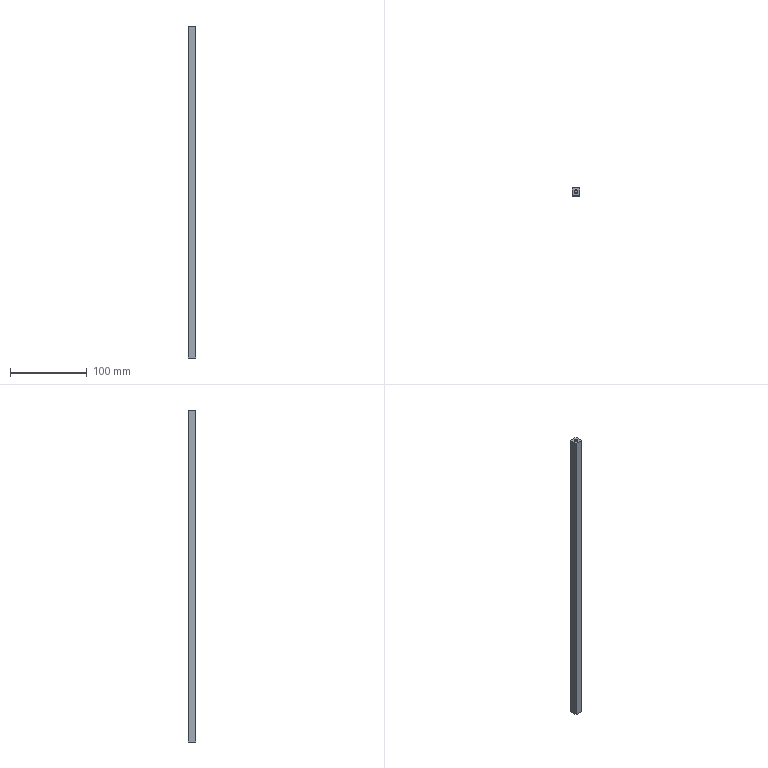Part | STEP file | End strip | 1 solid | 16 faces | box 10 x 10 x 432 mm | volume 42976 mm3 | plane 8 | cone 4 | cylinder 4 | commonest cylinder face diameters 3 x4
STEP:
#1=CARTESIAN_POINT('',(-16.382,-19.086,1.));
#2=VERTEX_POINT('',#1);
#3=CARTESIAN_POINT('',(-19.382,-19.086,1.));
#4=VERTEX_POINT('',#3);
#5=CARTESIAN_POINT('',(-17.882,-19.086,1.));
#6=DIRECTION('',(0.,0.,-1.));
#7=DIRECTION('',(-1.,0.,0.));
#8=AXIS2_PLACEMENT_3D('',#5,#6,#7);
#9=CIRCLE('',#8,1.5);
#10=EDGE_CURVE('',#2,#4,#9,.T.);
#11=ORIENTED_EDGE('',*,*,#10,.F.);
#12=CARTESIAN_POINT('',(-15.382,-19.086,0.));
#13=VERTEX_POINT('',#12);
#14=CARTESIAN_POINT('',(-15.382,-19.086,0.));
#15=DIRECTION('',(0.7071,0.,-0.7071));
#16=VECTOR('',#15,1000.);
#17=LINE('',#14,#16);
#18=EDGE_CURVE('',#2,#13,#17,.T.);
#19=ORIENTED_EDGE('',*,*,#18,.T.);
#20=CARTESIAN_POINT('',(-20.382,-19.086,0.));
#21=VERTEX_POINT('',#20);
#22=CARTESIAN_POINT('',(-17.882,-19.086,0.));
#23=DIRECTION('',(0.,0.,-1.));
#24=DIRECTION('',(-1.,0.,0.));
#25=AXIS2_PLACEMENT_3D('',#22,#23,#24);
#26=CIRCLE('',#25,2.5);
#27=EDGE_CURVE('',#13,#21,#26,.T.);
#28=ORIENTED_EDGE('',*,*,#27,.T.);
#29=CARTESIAN_POINT('',(-20.382,-19.086,0.));
#30=DIRECTION('',(-0.7071,0.,-0.7071));
#31=VECTOR('',#30,1000.);
#32=LINE('',#29,#31);
#33=EDGE_CURVE('',#4,#21,#32,.T.);
#34=ORIENTED_EDGE('',*,*,#33,.F.);
#35=EDGE_LOOP('',(#11,#19,#28,#34));
#36=FACE_OUTER_BOUND('',#35,.T.);
#37=CARTESIAN_POINT('',(-17.882,-19.086,0.));
#38=DIRECTION('',(0.,0.,-1.));
#39=DIRECTION('',(-1.,0.,0.));
#40=AXIS2_PLACEMENT_3D('',#37,#38,#39);
#41=CONICAL_SURFACE('',#40,2.5,0.7854);
#42=ADVANCED_FACE('',(#36),#41,.F.);
#43=CARTESIAN_POINT('',(-17.882,-17.586,431.));
#44=VERTEX_POINT('',#43);
#45=CARTESIAN_POINT('',(-19.382,-19.086,431.));
#46=VERTEX_POINT('',#45);
#47=CARTESIAN_POINT('',(-17.882,-19.086,431.));
#48=DIRECTION('',(0.,0.,1.));
#49=DIRECTION('',(1.,0.,0.));
#50=AXIS2_PLACEMENT_3D('',#47,#48,#49);
#51=CIRCLE('',#50,1.5);
#52=EDGE_CURVE('',#44,#46,#51,.T.);
#53=ORIENTED_EDGE('',*,*,#52,.F.);
#54=CARTESIAN_POINT('',(-17.882,-16.586,432.));
#55=VERTEX_POINT('',#54);
#56=CARTESIAN_POINT('',(-17.882,-16.586,432.));
#57=DIRECTION('',(0.,0.7071,0.7071));
#58=VECTOR('',#57,1000.);
#59=LINE('',#56,#58);
#60=EDGE_CURVE('',#44,#55,#59,.T.);
#61=ORIENTED_EDGE('',*,*,#60,.T.);
#62=CARTESIAN_POINT('',(-17.882,-21.586,432.));
#63=VERTEX_POINT('',#62);
#64=CARTESIAN_POINT('',(-17.882,-19.086,432.));
#65=DIRECTION('',(0.,0.,-1.));
#66=DIRECTION('',(0.,-1.,0.));
#67=AXIS2_PLACEMENT_3D('',#64,#65,#66);
#68=CIRCLE('',#67,2.5);
#69=EDGE_CURVE('',#63,#55,#68,.T.);
#70=ORIENTED_EDGE('',*,*,#69,.F.);
#71=CARTESIAN_POINT('',(-17.882,-20.586,431.));
#72=VERTEX_POINT('',#71);
#73=CARTESIAN_POINT('',(-17.882,-21.586,432.));
#74=DIRECTION('',(0.,-0.7071,0.7071));
#75=VECTOR('',#74,1000.);
#76=LINE('',#73,#75);
#77=EDGE_CURVE('',#72,#63,#76,.T.);
#78=ORIENTED_EDGE('',*,*,#77,.F.);
#79=CARTESIAN_POINT('',(-17.882,-19.086,431.));
#80=DIRECTION('',(0.,0.,1.));
#81=DIRECTION('',(1.,0.,0.));
#82=AXIS2_PLACEMENT_3D('',#79,#80,#81);
#83=CIRCLE('',#82,1.5);
#84=EDGE_CURVE('',#46,#72,#83,.T.);
#85=ORIENTED_EDGE('',*,*,#84,.F.);
#86=EDGE_LOOP('',(#53,#61,#70,#78,#85));
#87=FACE_OUTER_BOUND('',#86,.T.);
#88=CARTESIAN_POINT('',(-17.882,-19.086,432.));
#89=DIRECTION('',(0.,0.,1.));
#90=DIRECTION('',(0.,-1.,0.));
#91=AXIS2_PLACEMENT_3D('',#88,#89,#90);
#92=CONICAL_SURFACE('',#91,2.5,0.7854);
#93=ADVANCED_FACE('',(#87),#92,.F.);
#94=CARTESIAN_POINT('',(-16.382,-19.086,15.));
#95=VERTEX_POINT('',#94);
#96=CARTESIAN_POINT('',(-19.382,-19.086,15.));
#97=VERTEX_POINT('',#96);
#98=CARTESIAN_POINT('',(-17.882,-19.086,15.));
#99=DIRECTION('',(0.,0.,-1.));
#100=DIRECTION('',(-1.,0.,0.));
#101=AXIS2_PLACEMENT_3D('',#98,#99,#100);
#102=CIRCLE('',#101,1.5);
#103=EDGE_CURVE('',#95,#97,#102,.T.);
#104=ORIENTED_EDGE('',*,*,#103,.F.);
#105=CARTESIAN_POINT('',(-16.382,-19.086,15.));
#106=DIRECTION('',(0.,0.,-1.));
#107=VECTOR('',#106,1000.);
#108=LINE('',#105,#107);
#109=EDGE_CURVE('',#95,#2,#108,.T.);
#110=ORIENTED_EDGE('',*,*,#109,.T.);
#111=ORIENTED_EDGE('',*,*,#10,.T.);
#112=CARTESIAN_POINT('',(-19.382,-19.086,15.));
#113=DIRECTION('',(0.,0.,-1.));
#114=VECTOR('',#113,1000.);
#115=LINE('',#112,#114);
#116=EDGE_CURVE('',#97,#4,#115,.T.);
#117=ORIENTED_EDGE('',*,*,#116,.F.);
#118=EDGE_LOOP('',(#104,#110,#111,#117));
#119=FACE_OUTER_BOUND('',#118,.T.);
#120=CARTESIAN_POINT('',(-17.882,-19.086,15.));
#121=DIRECTION('',(0.,0.,-1.));
#122=DIRECTION('',(-1.,0.,0.));
#123=AXIS2_PLACEMENT_3D('',#120,#121,#122);
#124=CYLINDRICAL_SURFACE('',#123,1.5);
#125=ADVANCED_FACE('',(#119),#124,.F.);
#126=CARTESIAN_POINT('',(-19.382,-19.086,417.));
#127=VERTEX_POINT('',#126);
#128=CARTESIAN_POINT('',(-16.382,-19.086,417.));
#129=VERTEX_POINT('',#128);
#130=CARTESIAN_POINT('',(-17.882,-19.086,417.));
#131=DIRECTION('',(0.,0.,1.));
#132=DIRECTION('',(1.,0.,0.));
#133=AXIS2_PLACEMENT_3D('',#130,#131,#132);
#134=CIRCLE('',#133,1.5);
#135=EDGE_CURVE('',#127,#129,#134,.T.);
#136=ORIENTED_EDGE('',*,*,#135,.F.);
#137=CARTESIAN_POINT('',(-19.382,-19.086,417.));
#138=DIRECTION('',(0.,0.,1.));
#139=VECTOR('',#138,1000.);
#140=LINE('',#137,#139);
#141=EDGE_CURVE('',#127,#46,#140,.T.);
#142=ORIENTED_EDGE('',*,*,#141,.T.);
#143=ORIENTED_EDGE('',*,*,#84,.T.);
#144=CARTESIAN_POINT('',(-16.382,-19.086,431.));
#145=VERTEX_POINT('',#144);
#146=CARTESIAN_POINT('',(-17.882,-19.086,431.));
#147=DIRECTION('',(0.,0.,1.));
#148=DIRECTION('',(1.,0.,0.));
#149=AXIS2_PLACEMENT_3D('',#146,#147,#148);
#150=CIRCLE('',#149,1.5);
#151=EDGE_CURVE('',#72,#145,#150,.T.);
#152=ORIENTED_EDGE('',*,*,#151,.T.);
#153=CARTESIAN_POINT('',(-16.382,-19.086,417.));
#154=DIRECTION('',(0.,0.,1.));
#155=VECTOR('',#154,1000.);
#156=LINE('',#153,#155);
#157=EDGE_CURVE('',#129,#145,#156,.T.);
#158=ORIENTED_EDGE('',*,*,#157,.F.);
#159=EDGE_LOOP('',(#136,#142,#143,#152,#158));
#160=FACE_OUTER_BOUND('',#159,.T.);
#161=CARTESIAN_POINT('',(-17.882,-19.086,417.));
#162=DIRECTION('',(0.,0.,1.));
#163=DIRECTION('',(1.,0.,0.));
#164=AXIS2_PLACEMENT_3D('',#161,#162,#163);
#165=CYLINDRICAL_SURFACE('',#164,1.5);
#166=ADVANCED_FACE('',(#160),#165,.F.);
#167=CARTESIAN_POINT('',(-22.882,-24.086,432.));
#168=VERTEX_POINT('',#167);
#169=CARTESIAN_POINT('',(-22.882,-24.086,0.));
#170=VERTEX_POINT('',#169);
#171=CARTESIAN_POINT('',(-22.882,-24.086,432.));
#172=DIRECTION('',(0.,0.,-1.));
#173=VECTOR('',#172,1000.);
#174=LINE('',#171,#173);
#175=EDGE_CURVE('',#168,#170,#174,.T.);
#176=ORIENTED_EDGE('',*,*,#175,.F.);
#177=CARTESIAN_POINT('',(-22.882,-14.086,432.));
#178=VERTEX_POINT('',#177);
#179=CARTESIAN_POINT('',(-22.882,-14.086,432.));
#180=DIRECTION('',(0.,-1.,0.));
#181=VECTOR('',#180,1000.);
#182=LINE('',#179,#181);
#183=EDGE_CURVE('',#178,#168,#182,.T.);
#184=ORIENTED_EDGE('',*,*,#183,.F.);
#185=CARTESIAN_POINT('',(-22.882,-14.086,0.));
#186=VERTEX_POINT('',#185);
#187=CARTESIAN_POINT('',(-22.882,-14.086,432.));
#188=DIRECTION('',(0.,0.,1.));
#189=VECTOR('',#188,1000.);
#190=LINE('',#187,#189);
#191=EDGE_CURVE('',#186,#178,#190,.T.);
#192=ORIENTED_EDGE('',*,*,#191,.F.);
#193=CARTESIAN_POINT('',(-22.882,-14.086,0.));
#194=DIRECTION('',(0.,1.,0.));
#195=VECTOR('',#194,1000.);
#196=LINE('',#193,#195);
#197=EDGE_CURVE('',#170,#186,#196,.T.);
#198=ORIENTED_EDGE('',*,*,#197,.F.);
#199=EDGE_LOOP('',(#176,#184,#192,#198));
#200=FACE_OUTER_BOUND('',#199,.T.);
#201=CARTESIAN_POINT('',(-22.882,-14.086,432.));
#202=DIRECTION('',(1.,0.,0.));
#203=DIRECTION('',(0.,0.,-1.));
#204=AXIS2_PLACEMENT_3D('',#201,#202,#203);
#205=PLANE('',#204);
#206=ADVANCED_FACE('',(#200),#205,.F.);
#207=CARTESIAN_POINT('',(-12.882,-14.086,0.));
#208=VERTEX_POINT('',#207);
#209=CARTESIAN_POINT('',(-22.882,-14.086,0.));
#210=DIRECTION('',(-1.,0.,0.));
#211=VECTOR('',#210,1000.);
#212=LINE('',#209,#211);
#213=EDGE_CURVE('',#208,#186,#212,.T.);
#214=ORIENTED_EDGE('',*,*,#213,.F.);
#215=CARTESIAN_POINT('',(-12.882,-24.086,0.));
#216=VERTEX_POINT('',#215);
#217=CARTESIAN_POINT('',(-12.882,-24.086,0.));
#218=DIRECTION('',(0.,1.,0.));
#219=VECTOR('',#218,1000.);
#220=LINE('',#217,#219);
#221=EDGE_CURVE('',#216,#208,#220,.T.);
#222=ORIENTED_EDGE('',*,*,#221,.F.);
#223=CARTESIAN_POINT('',(-22.882,-24.086,0.));
#224=DIRECTION('',(1.,0.,0.));
#225=VECTOR('',#224,1000.);
#226=LINE('',#223,#225);
#227=EDGE_CURVE('',#170,#216,#226,.T.);
#228=ORIENTED_EDGE('',*,*,#227,.F.);
#229=ORIENTED_EDGE('',*,*,#197,.T.);
#230=EDGE_LOOP('',(#214,#222,#228,#229));
#231=FACE_OUTER_BOUND('',#230,.T.);
#232=CARTESIAN_POINT('',(-17.882,-19.086,0.));
#233=DIRECTION('',(0.,0.,-1.));
#234=DIRECTION('',(-1.,0.,0.));
#235=AXIS2_PLACEMENT_3D('',#232,#233,#234);
#236=CIRCLE('',#235,2.5);
#237=EDGE_CURVE('',#21,#13,#236,.T.);
#238=ORIENTED_EDGE('',*,*,#237,.F.);
#239=ORIENTED_EDGE('',*,*,#27,.F.);
#240=EDGE_LOOP('',(#238,#239));
#241=FACE_BOUND('',#240,.T.);
#242=CARTESIAN_POINT('',(-22.882,-24.086,0.));
#243=DIRECTION('',(0.,0.,1.));
#244=DIRECTION('',(1.,0.,0.));
#245=AXIS2_PLACEMENT_3D('',#242,#243,#244);
#246=PLANE('',#245);
#247=ADVANCED_FACE('',(#231,#241),#246,.F.);
#248=CARTESIAN_POINT('',(-12.882,-24.086,432.));
#249=VERTEX_POINT('',#248);
#250=CARTESIAN_POINT('',(-12.882,-24.086,432.));
#251=DIRECTION('',(0.,0.,-1.));
#252=VECTOR('',#251,1000.);
#253=LINE('',#250,#252);
#254=EDGE_CURVE('',#249,#216,#253,.T.);
#255=ORIENTED_EDGE('',*,*,#254,.F.);
#256=CARTESIAN_POINT('',(-22.882,-24.086,432.));
#257=DIRECTION('',(1.,0.,0.));
#258=VECTOR('',#257,1000.);
#259=LINE('',#256,#258);
#260=EDGE_CURVE('',#168,#249,#259,.T.);
#261=ORIENTED_EDGE('',*,*,#260,.F.);
#262=ORIENTED_EDGE('',*,*,#175,.T.);
#263=ORIENTED_EDGE('',*,*,#227,.T.);
#264=EDGE_LOOP('',(#255,#261,#262,#263));
#265=FACE_OUTER_BOUND('',#264,.T.);
#266=CARTESIAN_POINT('',(-22.882,-24.086,432.));
#267=DIRECTION('',(0.,1.,0.));
#268=DIRECTION('',(0.,0.,1.));
#269=AXIS2_PLACEMENT_3D('',#266,#267,#268);
#270=PLANE('',#269);
#271=ADVANCED_FACE('',(#265),#270,.F.);
#272=CARTESIAN_POINT('',(-12.882,-14.086,432.));
#273=VERTEX_POINT('',#272);
#274=CARTESIAN_POINT('',(-12.882,-24.086,432.));
#275=DIRECTION('',(0.,1.,0.));
#276=VECTOR('',#275,1000.);
#277=LINE('',#274,#276);
#278=EDGE_CURVE('',#249,#273,#277,.T.);
#279=ORIENTED_EDGE('',*,*,#278,.T.);
#280=CARTESIAN_POINT('',(-22.882,-14.086,432.));
#281=DIRECTION('',(-1.,0.,0.));
#282=VECTOR('',#281,1000.);
#283=LINE('',#280,#282);
#284=EDGE_CURVE('',#273,#178,#283,.T.);
#285=ORIENTED_EDGE('',*,*,#284,.T.);
#286=ORIENTED_EDGE('',*,*,#183,.T.);
#287=ORIENTED_EDGE('',*,*,#260,.T.);
#288=EDGE_LOOP('',(#279,#285,#286,#287));
#289=FACE_OUTER_BOUND('',#288,.T.);
#290=ORIENTED_EDGE('',*,*,#69,.T.);
#291=CARTESIAN_POINT('',(-17.882,-19.086,432.));
#292=DIRECTION('',(0.,0.,-1.));
#293=DIRECTION('',(0.,-1.,0.));
#294=AXIS2_PLACEMENT_3D('',#291,#292,#293);
#295=CIRCLE('',#294,2.5);
#296=EDGE_CURVE('',#55,#63,#295,.T.);
#297=ORIENTED_EDGE('',*,*,#296,.T.);
#298=EDGE_LOOP('',(#290,#297));
#299=FACE_BOUND('',#298,.T.);
#300=CARTESIAN_POINT('',(-22.882,-24.086,432.));
#301=DIRECTION('',(0.,0.,1.));
#302=DIRECTION('',(1.,0.,0.));
#303=AXIS2_PLACEMENT_3D('',#300,#301,#302);
#304=PLANE('',#303);
#305=ADVANCED_FACE('',(#289,#299),#304,.T.);
#306=ORIENTED_EDGE('',*,*,#191,.T.);
#307=ORIENTED_EDGE('',*,*,#284,.F.);
#308=CARTESIAN_POINT('',(-12.882,-14.086,432.));
#309=DIRECTION('',(0.,0.,1.));
#310=VECTOR('',#309,1000.);
#311=LINE('',#308,#310);
#312=EDGE_CURVE('',#208,#273,#311,.T.);
#313=ORIENTED_EDGE('',*,*,#312,.F.);
#314=ORIENTED_EDGE('',*,*,#213,.T.);
#315=EDGE_LOOP('',(#306,#307,#313,#314));
#316=FACE_OUTER_BOUND('',#315,.T.);
#317=CARTESIAN_POINT('',(-22.882,-14.086,432.));
#318=DIRECTION('',(0.,-1.,0.));
#319=DIRECTION('',(0.,0.,-1.));
#320=AXIS2_PLACEMENT_3D('',#317,#318,#319);
#321=PLANE('',#320);
#322=ADVANCED_FACE('',(#316),#321,.F.);
#323=ORIENTED_EDGE('',*,*,#312,.T.);
#324=ORIENTED_EDGE('',*,*,#278,.F.);
#325=ORIENTED_EDGE('',*,*,#254,.T.);
#326=ORIENTED_EDGE('',*,*,#221,.T.);
#327=EDGE_LOOP('',(#323,#324,#325,#326));
#328=FACE_OUTER_BOUND('',#327,.T.);
#329=CARTESIAN_POINT('',(-12.882,-14.086,432.));
#330=DIRECTION('',(-1.,0.,0.));
#331=DIRECTION('',(0.,-1.,0.));
#332=AXIS2_PLACEMENT_3D('',#329,#330,#331);
#333=PLANE('',#332);
#334=ADVANCED_FACE('',(#328),#333,.F.);
#335=ORIENTED_EDGE('',*,*,#18,.F.);
#336=CARTESIAN_POINT('',(-17.882,-19.086,1.));
#337=DIRECTION('',(0.,0.,-1.));
#338=DIRECTION('',(-1.,0.,0.));
#339=AXIS2_PLACEMENT_3D('',#336,#337,#338);
#340=CIRCLE('',#339,1.5);
#341=EDGE_CURVE('',#4,#2,#340,.T.);
#342=ORIENTED_EDGE('',*,*,#341,.F.);
#343=ORIENTED_EDGE('',*,*,#33,.T.);
#344=ORIENTED_EDGE('',*,*,#237,.T.);
#345=EDGE_LOOP('',(#335,#342,#343,#344));
#346=FACE_OUTER_BOUND('',#345,.T.);
#347=CARTESIAN_POINT('',(-17.882,-19.086,0.));
#348=DIRECTION('',(0.,0.,-1.));
#349=DIRECTION('',(-1.,0.,0.));
#350=AXIS2_PLACEMENT_3D('',#347,#348,#349);
#351=CONICAL_SURFACE('',#350,2.5,0.7854);
#352=ADVANCED_FACE('',(#346),#351,.F.);
#353=ORIENTED_EDGE('',*,*,#60,.F.);
#354=CARTESIAN_POINT('',(-17.882,-19.086,431.));
#355=DIRECTION('',(0.,0.,1.));
#356=DIRECTION('',(1.,0.,0.));
#357=AXIS2_PLACEMENT_3D('',#354,#355,#356);
#358=CIRCLE('',#357,1.5);
#359=EDGE_CURVE('',#145,#44,#358,.T.);
#360=ORIENTED_EDGE('',*,*,#359,.F.);
#361=ORIENTED_EDGE('',*,*,#151,.F.);
#362=ORIENTED_EDGE('',*,*,#77,.T.);
#363=ORIENTED_EDGE('',*,*,#296,.F.);
#364=EDGE_LOOP('',(#353,#360,#361,#362,#363));
#365=FACE_OUTER_BOUND('',#364,.T.);
#366=CARTESIAN_POINT('',(-17.882,-19.086,432.));
#367=DIRECTION('',(0.,0.,1.));
#368=DIRECTION('',(0.,-1.,0.));
#369=AXIS2_PLACEMENT_3D('',#366,#367,#368);
#370=CONICAL_SURFACE('',#369,2.5,0.7854);
#371=ADVANCED_FACE('',(#365),#370,.F.);
#372=ORIENTED_EDGE('',*,*,#109,.F.);
#373=CARTESIAN_POINT('',(-17.882,-19.086,15.));
#374=DIRECTION('',(0.,0.,-1.));
#375=DIRECTION('',(-1.,0.,0.));
#376=AXIS2_PLACEMENT_3D('',#373,#374,#375);
#377=CIRCLE('',#376,1.5);
#378=EDGE_CURVE('',#97,#95,#377,.T.);
#379=ORIENTED_EDGE('',*,*,#378,.F.);
#380=ORIENTED_EDGE('',*,*,#116,.T.);
#381=ORIENTED_EDGE('',*,*,#341,.T.);
#382=EDGE_LOOP('',(#372,#379,#380,#381));
#383=FACE_OUTER_BOUND('',#382,.T.);
#384=CARTESIAN_POINT('',(-17.882,-19.086,15.));
#385=DIRECTION('',(0.,0.,-1.));
#386=DIRECTION('',(-1.,0.,0.));
#387=AXIS2_PLACEMENT_3D('',#384,#385,#386);
#388=CYLINDRICAL_SURFACE('',#387,1.5);
#389=ADVANCED_FACE('',(#383),#388,.F.);
#390=ORIENTED_EDGE('',*,*,#141,.F.);
#391=CARTESIAN_POINT('',(-17.882,-19.086,417.));
#392=DIRECTION('',(0.,0.,1.));
#393=DIRECTION('',(1.,0.,0.));
#394=AXIS2_PLACEMENT_3D('',#391,#392,#393);
#395=CIRCLE('',#394,1.5);
#396=EDGE_CURVE('',#129,#127,#395,.T.);
#397=ORIENTED_EDGE('',*,*,#396,.F.);
#398=ORIENTED_EDGE('',*,*,#157,.T.);
#399=ORIENTED_EDGE('',*,*,#359,.T.);
#400=ORIENTED_EDGE('',*,*,#52,.T.);
#401=EDGE_LOOP('',(#390,#397,#398,#399,#400));
#402=FACE_OUTER_BOUND('',#401,.T.);
#403=CARTESIAN_POINT('',(-17.882,-19.086,417.));
#404=DIRECTION('',(0.,0.,1.));
#405=DIRECTION('',(1.,0.,0.));
#406=AXIS2_PLACEMENT_3D('',#403,#404,#405);
#407=CYLINDRICAL_SURFACE('',#406,1.5);
#408=ADVANCED_FACE('',(#402),#407,.F.);
#409=ORIENTED_EDGE('',*,*,#378,.T.);
#410=ORIENTED_EDGE('',*,*,#103,.T.);
#411=EDGE_LOOP('',(#409,#410));
#412=FACE_OUTER_BOUND('',#411,.T.);
#413=CARTESIAN_POINT('',(-17.882,-19.086,15.));
#414=DIRECTION('',(0.,0.,-1.));
#415=DIRECTION('',(-1.,0.,0.));
#416=AXIS2_PLACEMENT_3D('',#413,#414,#415);
#417=PLANE('',#416);
#418=ADVANCED_FACE('',(#412),#417,.T.);
#419=ORIENTED_EDGE('',*,*,#396,.T.);
#420=ORIENTED_EDGE('',*,*,#135,.T.);
#421=EDGE_LOOP('',(#419,#420));
#422=FACE_OUTER_BOUND('',#421,.T.);
#423=CARTESIAN_POINT('',(-17.882,-19.086,417.));
#424=DIRECTION('',(0.,0.,1.));
#425=DIRECTION('',(1.,0.,0.));
#426=AXIS2_PLACEMENT_3D('',#423,#424,#425);
#427=PLANE('',#426);
#428=ADVANCED_FACE('',(#422),#427,.T.);
#429=CLOSED_SHELL('',(#42,#93,#125,#166,#206,#247,#271,#305,#322,#334,#352,#371,#389,#408,#418,#428));
#430=MANIFOLD_SOLID_BREP('',#429);
#431=CARTESIAN_POINT('',(0.,0.,0.));
#432=DIRECTION('',(0.,0.,1.));
#433=DIRECTION('',(1.,0.,0.));
#434=AXIS2_PLACEMENT_3D('',#431,#432,#433);
#435=(LENGTH_UNIT()NAMED_UNIT(*)SI_UNIT(.MILLI.,.METRE.));
#436=UNCERTAINTY_MEASURE_WITH_UNIT(LENGTH_MEASURE(0.00001),#435,'','');
#437=(NAMED_UNIT(*)PLANE_ANGLE_UNIT()SI_UNIT($,.RADIAN.));
#438=(NAMED_UNIT(*)SI_UNIT($,.STERADIAN.)SOLID_ANGLE_UNIT());
#439=(GEOMETRIC_REPRESENTATION_CONTEXT(3)GLOBAL_UNCERTAINTY_ASSIGNED_CONTEXT((#436))GLOBAL_UNIT_ASSIGNED_CONTEXT((#435,#437,#438))REPRESENTATION_CONTEXT('',''));
#440=ADVANCED_BREP_SHAPE_REPRESENTATION('',(#430,#434),#439);